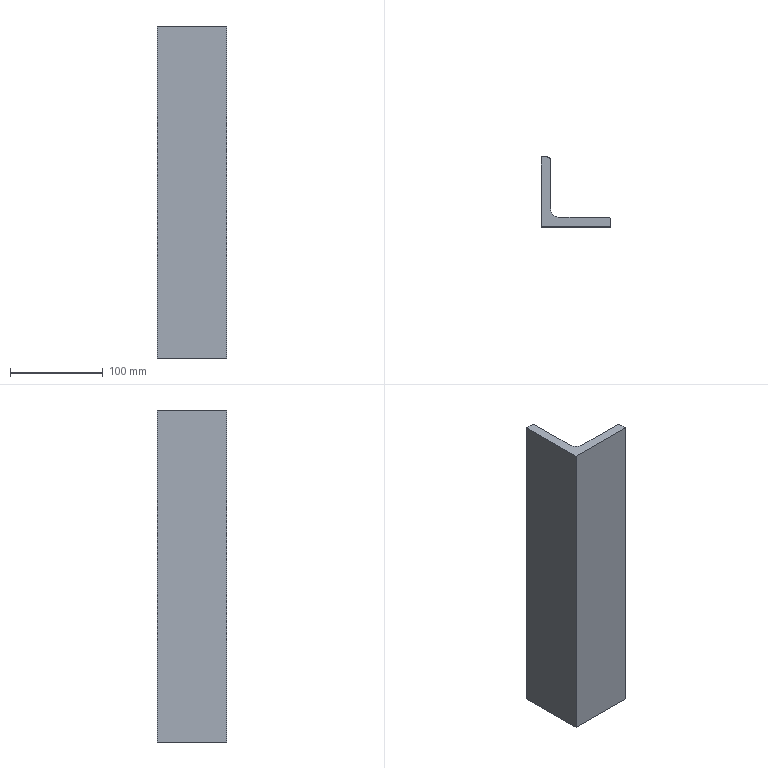Part | SolidWorks | features Extrusion 1 | 1 solid | 11 faces | box 75 x 75 x 358.1 mm | volume 505682 mm3 | plane 8 | cylinder 3 | commonest cylinder face diameters 7 x2 18 x1
STEP:
#1=CARTESIAN_POINT('',(6.5,75.,-179.05));
#2=VERTEX_POINT('',#1);
#3=CARTESIAN_POINT('',(0.,75.,-179.05));
#4=VERTEX_POINT('',#3);
#5=CARTESIAN_POINT('',(6.5,75.,-179.05));
#6=DIRECTION('',(-1.,0.,0.));
#7=VECTOR('',#6,1000.);
#8=LINE('',#5,#7);
#9=EDGE_CURVE('',#2,#4,#8,.T.);
#10=ORIENTED_EDGE('',*,*,#9,.T.);
#11=CARTESIAN_POINT('',(0.,75.,179.05));
#12=VERTEX_POINT('',#11);
#13=CARTESIAN_POINT('',(0.,75.,179.05));
#14=DIRECTION('',(0.,0.,-1.));
#15=VECTOR('',#14,1000.);
#16=LINE('',#13,#15);
#17=EDGE_CURVE('',#12,#4,#16,.T.);
#18=ORIENTED_EDGE('',*,*,#17,.F.);
#19=CARTESIAN_POINT('',(6.5,75.,179.05));
#20=VERTEX_POINT('',#19);
#21=CARTESIAN_POINT('',(6.5,75.,179.05));
#22=DIRECTION('',(-1.,0.,0.));
#23=VECTOR('',#22,1000.);
#24=LINE('',#21,#23);
#25=EDGE_CURVE('',#20,#12,#24,.T.);
#26=ORIENTED_EDGE('',*,*,#25,.F.);
#27=CARTESIAN_POINT('',(6.5,75.,179.05));
#28=DIRECTION('',(0.,0.,-1.));
#29=VECTOR('',#28,1000.);
#30=LINE('',#27,#29);
#31=EDGE_CURVE('',#20,#2,#30,.T.);
#32=ORIENTED_EDGE('',*,*,#31,.T.);
#33=EDGE_LOOP('',(#10,#18,#26,#32));
#34=FACE_OUTER_BOUND('',#33,.T.);
#35=CARTESIAN_POINT('',(6.5,75.,179.05));
#36=DIRECTION('',(0.,-1.,0.));
#37=DIRECTION('',(0.,0.,-1.));
#38=AXIS2_PLACEMENT_3D('',#35,#36,#37);
#39=PLANE('',#38);
#40=ADVANCED_FACE('',(#34),#39,.F.);
#41=CARTESIAN_POINT('',(0.,0.,-179.05));
#42=VERTEX_POINT('',#41);
#43=CARTESIAN_POINT('',(0.,75.,-179.05));
#44=DIRECTION('',(0.,-1.,0.));
#45=VECTOR('',#44,1000.);
#46=LINE('',#43,#45);
#47=EDGE_CURVE('',#4,#42,#46,.T.);
#48=ORIENTED_EDGE('',*,*,#47,.T.);
#49=CARTESIAN_POINT('',(0.,0.,179.05));
#50=VERTEX_POINT('',#49);
#51=CARTESIAN_POINT('',(0.,0.,179.05));
#52=DIRECTION('',(0.,0.,-1.));
#53=VECTOR('',#52,1000.);
#54=LINE('',#51,#53);
#55=EDGE_CURVE('',#50,#42,#54,.T.);
#56=ORIENTED_EDGE('',*,*,#55,.F.);
#57=CARTESIAN_POINT('',(0.,75.,179.05));
#58=DIRECTION('',(0.,-1.,0.));
#59=VECTOR('',#58,1000.);
#60=LINE('',#57,#59);
#61=EDGE_CURVE('',#12,#50,#60,.T.);
#62=ORIENTED_EDGE('',*,*,#61,.F.);
#63=ORIENTED_EDGE('',*,*,#17,.T.);
#64=EDGE_LOOP('',(#48,#56,#62,#63));
#65=FACE_OUTER_BOUND('',#64,.T.);
#66=CARTESIAN_POINT('',(0.,75.,179.05));
#67=DIRECTION('',(1.,0.,0.));
#68=DIRECTION('',(0.,1.,0.));
#69=AXIS2_PLACEMENT_3D('',#66,#67,#68);
#70=PLANE('',#69);
#71=ADVANCED_FACE('',(#65),#70,.F.);
#72=CARTESIAN_POINT('',(75.,0.,-179.05));
#73=VERTEX_POINT('',#72);
#74=CARTESIAN_POINT('',(0.,0.,-179.05));
#75=DIRECTION('',(1.,0.,0.));
#76=VECTOR('',#75,1000.);
#77=LINE('',#74,#76);
#78=EDGE_CURVE('',#42,#73,#77,.T.);
#79=ORIENTED_EDGE('',*,*,#78,.T.);
#80=CARTESIAN_POINT('',(75.,0.,179.05));
#81=VERTEX_POINT('',#80);
#82=CARTESIAN_POINT('',(75.,0.,179.05));
#83=DIRECTION('',(0.,0.,-1.));
#84=VECTOR('',#83,1000.);
#85=LINE('',#82,#84);
#86=EDGE_CURVE('',#81,#73,#85,.T.);
#87=ORIENTED_EDGE('',*,*,#86,.F.);
#88=CARTESIAN_POINT('',(0.,0.,179.05));
#89=DIRECTION('',(1.,0.,0.));
#90=VECTOR('',#89,1000.);
#91=LINE('',#88,#90);
#92=EDGE_CURVE('',#50,#81,#91,.T.);
#93=ORIENTED_EDGE('',*,*,#92,.F.);
#94=ORIENTED_EDGE('',*,*,#55,.T.);
#95=EDGE_LOOP('',(#79,#87,#93,#94));
#96=FACE_OUTER_BOUND('',#95,.T.);
#97=CARTESIAN_POINT('',(0.,0.,179.05));
#98=DIRECTION('',(0.,1.,0.));
#99=DIRECTION('',(0.,0.,1.));
#100=AXIS2_PLACEMENT_3D('',#97,#98,#99);
#101=PLANE('',#100);
#102=ADVANCED_FACE('',(#96),#101,.F.);
#103=CARTESIAN_POINT('',(75.,6.5,-179.05));
#104=VERTEX_POINT('',#103);
#105=CARTESIAN_POINT('',(75.,0.,-179.05));
#106=DIRECTION('',(0.,1.,0.));
#107=VECTOR('',#106,1000.);
#108=LINE('',#105,#107);
#109=EDGE_CURVE('',#73,#104,#108,.T.);
#110=ORIENTED_EDGE('',*,*,#109,.T.);
#111=CARTESIAN_POINT('',(75.,6.5,179.05));
#112=VERTEX_POINT('',#111);
#113=CARTESIAN_POINT('',(75.,6.5,179.05));
#114=DIRECTION('',(0.,0.,-1.));
#115=VECTOR('',#114,1000.);
#116=LINE('',#113,#115);
#117=EDGE_CURVE('',#112,#104,#116,.T.);
#118=ORIENTED_EDGE('',*,*,#117,.F.);
#119=CARTESIAN_POINT('',(75.,0.,179.05));
#120=DIRECTION('',(0.,1.,0.));
#121=VECTOR('',#120,1000.);
#122=LINE('',#119,#121);
#123=EDGE_CURVE('',#81,#112,#122,.T.);
#124=ORIENTED_EDGE('',*,*,#123,.F.);
#125=ORIENTED_EDGE('',*,*,#86,.T.);
#126=EDGE_LOOP('',(#110,#118,#124,#125));
#127=FACE_OUTER_BOUND('',#126,.T.);
#128=CARTESIAN_POINT('',(75.,0.,179.05));
#129=DIRECTION('',(-1.,0.,0.));
#130=DIRECTION('',(0.,0.,1.));
#131=AXIS2_PLACEMENT_3D('',#128,#129,#130);
#132=PLANE('',#131);
#133=ADVANCED_FACE('',(#127),#132,.F.);
#134=CARTESIAN_POINT('',(71.5,10.,-179.05));
#135=VERTEX_POINT('',#134);
#136=CARTESIAN_POINT('',(71.5,6.5,-179.05));
#137=DIRECTION('',(0.,0.,1.));
#138=DIRECTION('',(1.,0.,0.));
#139=AXIS2_PLACEMENT_3D('',#136,#137,#138);
#140=CIRCLE('',#139,3.5);
#141=EDGE_CURVE('',#104,#135,#140,.T.);
#142=ORIENTED_EDGE('',*,*,#141,.T.);
#143=CARTESIAN_POINT('',(71.5,10.,179.05));
#144=VERTEX_POINT('',#143);
#145=CARTESIAN_POINT('',(71.5,10.,179.05));
#146=DIRECTION('',(0.,0.,-1.));
#147=VECTOR('',#146,1000.);
#148=LINE('',#145,#147);
#149=EDGE_CURVE('',#144,#135,#148,.T.);
#150=ORIENTED_EDGE('',*,*,#149,.F.);
#151=CARTESIAN_POINT('',(71.5,6.5,179.05));
#152=DIRECTION('',(0.,0.,1.));
#153=DIRECTION('',(1.,0.,0.));
#154=AXIS2_PLACEMENT_3D('',#151,#152,#153);
#155=CIRCLE('',#154,3.5);
#156=EDGE_CURVE('',#112,#144,#155,.T.);
#157=ORIENTED_EDGE('',*,*,#156,.F.);
#158=ORIENTED_EDGE('',*,*,#117,.T.);
#159=EDGE_LOOP('',(#142,#150,#157,#158));
#160=FACE_OUTER_BOUND('',#159,.T.);
#161=CARTESIAN_POINT('',(71.5,6.5,179.05));
#162=DIRECTION('',(0.,0.,-1.));
#163=DIRECTION('',(-1.,0.,0.));
#164=AXIS2_PLACEMENT_3D('',#161,#162,#163);
#165=CYLINDRICAL_SURFACE('',#164,3.5);
#166=ADVANCED_FACE('',(#160),#165,.T.);
#167=CARTESIAN_POINT('',(19.,10.,-179.05));
#168=VERTEX_POINT('',#167);
#169=CARTESIAN_POINT('',(71.5,10.,-179.05));
#170=DIRECTION('',(-1.,0.,0.));
#171=VECTOR('',#170,1000.);
#172=LINE('',#169,#171);
#173=EDGE_CURVE('',#135,#168,#172,.T.);
#174=ORIENTED_EDGE('',*,*,#173,.T.);
#175=CARTESIAN_POINT('',(19.,10.,179.05));
#176=VERTEX_POINT('',#175);
#177=CARTESIAN_POINT('',(19.,10.,179.05));
#178=DIRECTION('',(0.,0.,-1.));
#179=VECTOR('',#178,1000.);
#180=LINE('',#177,#179);
#181=EDGE_CURVE('',#176,#168,#180,.T.);
#182=ORIENTED_EDGE('',*,*,#181,.F.);
#183=CARTESIAN_POINT('',(71.5,10.,179.05));
#184=DIRECTION('',(-1.,0.,0.));
#185=VECTOR('',#184,1000.);
#186=LINE('',#183,#185);
#187=EDGE_CURVE('',#144,#176,#186,.T.);
#188=ORIENTED_EDGE('',*,*,#187,.F.);
#189=ORIENTED_EDGE('',*,*,#149,.T.);
#190=EDGE_LOOP('',(#174,#182,#188,#189));
#191=FACE_OUTER_BOUND('',#190,.T.);
#192=CARTESIAN_POINT('',(71.5,10.,179.05));
#193=DIRECTION('',(0.,-1.,0.));
#194=DIRECTION('',(1.,0.,0.));
#195=AXIS2_PLACEMENT_3D('',#192,#193,#194);
#196=PLANE('',#195);
#197=ADVANCED_FACE('',(#191),#196,.F.);
#198=CARTESIAN_POINT('',(10.,19.,-179.05));
#199=VERTEX_POINT('',#198);
#200=CARTESIAN_POINT('',(19.,19.,-179.05));
#201=DIRECTION('',(0.,0.,-1.));
#202=DIRECTION('',(-1.,0.,0.));
#203=AXIS2_PLACEMENT_3D('',#200,#201,#202);
#204=CIRCLE('',#203,9.);
#205=EDGE_CURVE('',#168,#199,#204,.T.);
#206=ORIENTED_EDGE('',*,*,#205,.T.);
#207=CARTESIAN_POINT('',(10.,19.,179.05));
#208=VERTEX_POINT('',#207);
#209=CARTESIAN_POINT('',(10.,19.,179.05));
#210=DIRECTION('',(0.,0.,-1.));
#211=VECTOR('',#210,1000.);
#212=LINE('',#209,#211);
#213=EDGE_CURVE('',#208,#199,#212,.T.);
#214=ORIENTED_EDGE('',*,*,#213,.F.);
#215=CARTESIAN_POINT('',(19.,19.,179.05));
#216=DIRECTION('',(0.,0.,-1.));
#217=DIRECTION('',(-1.,0.,0.));
#218=AXIS2_PLACEMENT_3D('',#215,#216,#217);
#219=CIRCLE('',#218,9.);
#220=EDGE_CURVE('',#176,#208,#219,.T.);
#221=ORIENTED_EDGE('',*,*,#220,.F.);
#222=ORIENTED_EDGE('',*,*,#181,.T.);
#223=EDGE_LOOP('',(#206,#214,#221,#222));
#224=FACE_OUTER_BOUND('',#223,.T.);
#225=CARTESIAN_POINT('',(19.,19.,179.05));
#226=DIRECTION('',(0.,0.,-1.));
#227=DIRECTION('',(-1.,0.,0.));
#228=AXIS2_PLACEMENT_3D('',#225,#226,#227);
#229=CYLINDRICAL_SURFACE('',#228,9.);
#230=ADVANCED_FACE('',(#224),#229,.F.);
#231=CARTESIAN_POINT('',(10.,71.5,-179.05));
#232=VERTEX_POINT('',#231);
#233=CARTESIAN_POINT('',(10.,19.,-179.05));
#234=DIRECTION('',(0.,1.,0.));
#235=VECTOR('',#234,1000.);
#236=LINE('',#233,#235);
#237=EDGE_CURVE('',#199,#232,#236,.T.);
#238=ORIENTED_EDGE('',*,*,#237,.T.);
#239=CARTESIAN_POINT('',(10.,71.5,179.05));
#240=VERTEX_POINT('',#239);
#241=CARTESIAN_POINT('',(10.,71.5,179.05));
#242=DIRECTION('',(0.,0.,-1.));
#243=VECTOR('',#242,1000.);
#244=LINE('',#241,#243);
#245=EDGE_CURVE('',#240,#232,#244,.T.);
#246=ORIENTED_EDGE('',*,*,#245,.F.);
#247=CARTESIAN_POINT('',(10.,19.,179.05));
#248=DIRECTION('',(0.,1.,0.));
#249=VECTOR('',#248,1000.);
#250=LINE('',#247,#249);
#251=EDGE_CURVE('',#208,#240,#250,.T.);
#252=ORIENTED_EDGE('',*,*,#251,.F.);
#253=ORIENTED_EDGE('',*,*,#213,.T.);
#254=EDGE_LOOP('',(#238,#246,#252,#253));
#255=FACE_OUTER_BOUND('',#254,.T.);
#256=CARTESIAN_POINT('',(10.,19.,179.05));
#257=DIRECTION('',(-1.,0.,0.));
#258=DIRECTION('',(0.,-1.,0.));
#259=AXIS2_PLACEMENT_3D('',#256,#257,#258);
#260=PLANE('',#259);
#261=ADVANCED_FACE('',(#255),#260,.F.);
#262=CARTESIAN_POINT('',(6.5,71.5,-179.05));
#263=DIRECTION('',(0.,0.,1.));
#264=DIRECTION('',(1.,0.,0.));
#265=AXIS2_PLACEMENT_3D('',#262,#263,#264);
#266=CIRCLE('',#265,3.5);
#267=EDGE_CURVE('',#232,#2,#266,.T.);
#268=ORIENTED_EDGE('',*,*,#267,.T.);
#269=ORIENTED_EDGE('',*,*,#31,.F.);
#270=CARTESIAN_POINT('',(6.5,71.5,179.05));
#271=DIRECTION('',(0.,0.,1.));
#272=DIRECTION('',(1.,0.,0.));
#273=AXIS2_PLACEMENT_3D('',#270,#271,#272);
#274=CIRCLE('',#273,3.5);
#275=EDGE_CURVE('',#240,#20,#274,.T.);
#276=ORIENTED_EDGE('',*,*,#275,.F.);
#277=ORIENTED_EDGE('',*,*,#245,.T.);
#278=EDGE_LOOP('',(#268,#269,#276,#277));
#279=FACE_OUTER_BOUND('',#278,.T.);
#280=CARTESIAN_POINT('',(6.5,71.5,179.05));
#281=DIRECTION('',(0.,0.,-1.));
#282=DIRECTION('',(-1.,0.,0.));
#283=AXIS2_PLACEMENT_3D('',#280,#281,#282);
#284=CYLINDRICAL_SURFACE('',#283,3.5);
#285=ADVANCED_FACE('',(#279),#284,.T.);
#286=ORIENTED_EDGE('',*,*,#25,.T.);
#287=ORIENTED_EDGE('',*,*,#61,.T.);
#288=ORIENTED_EDGE('',*,*,#92,.T.);
#289=ORIENTED_EDGE('',*,*,#123,.T.);
#290=ORIENTED_EDGE('',*,*,#156,.T.);
#291=ORIENTED_EDGE('',*,*,#187,.T.);
#292=ORIENTED_EDGE('',*,*,#220,.T.);
#293=ORIENTED_EDGE('',*,*,#251,.T.);
#294=ORIENTED_EDGE('',*,*,#275,.T.);
#295=EDGE_LOOP('',(#286,#287,#288,#289,#290,#291,#292,#293,#294));
#296=FACE_OUTER_BOUND('',#295,.T.);
#297=CARTESIAN_POINT('',(71.5,6.5,179.05));
#298=DIRECTION('',(0.,0.,1.));
#299=DIRECTION('',(1.,0.,0.));
#300=AXIS2_PLACEMENT_3D('',#297,#298,#299);
#301=PLANE('',#300);
#302=ADVANCED_FACE('',(#296),#301,.T.);
#303=ORIENTED_EDGE('',*,*,#9,.F.);
#304=ORIENTED_EDGE('',*,*,#267,.F.);
#305=ORIENTED_EDGE('',*,*,#237,.F.);
#306=ORIENTED_EDGE('',*,*,#205,.F.);
#307=ORIENTED_EDGE('',*,*,#173,.F.);
#308=ORIENTED_EDGE('',*,*,#141,.F.);
#309=ORIENTED_EDGE('',*,*,#109,.F.);
#310=ORIENTED_EDGE('',*,*,#78,.F.);
#311=ORIENTED_EDGE('',*,*,#47,.F.);
#312=EDGE_LOOP('',(#303,#304,#305,#306,#307,#308,#309,#310,#311));
#313=FACE_OUTER_BOUND('',#312,.T.);
#314=CARTESIAN_POINT('',(71.5,6.5,-179.05));
#315=DIRECTION('',(0.,0.,1.));
#316=DIRECTION('',(1.,0.,0.));
#317=AXIS2_PLACEMENT_3D('',#314,#315,#316);
#318=PLANE('',#317);
#319=ADVANCED_FACE('',(#313),#318,.F.);
#320=CLOSED_SHELL('',(#40,#71,#102,#133,#166,#197,#230,#261,#285,#302,#319));
#321=MANIFOLD_SOLID_BREP('',#320);
#322=CARTESIAN_POINT('',(0.,0.,0.));
#323=DIRECTION('',(0.,0.,1.));
#324=DIRECTION('',(1.,0.,0.));
#325=AXIS2_PLACEMENT_3D('',#322,#323,#324);
#326=(LENGTH_UNIT()NAMED_UNIT(*)SI_UNIT(.MILLI.,.METRE.));
#327=UNCERTAINTY_MEASURE_WITH_UNIT(LENGTH_MEASURE(0.00001),#326,'','');
#328=(NAMED_UNIT(*)PLANE_ANGLE_UNIT()SI_UNIT($,.RADIAN.));
#329=(NAMED_UNIT(*)SI_UNIT($,.STERADIAN.)SOLID_ANGLE_UNIT());
#330=(GEOMETRIC_REPRESENTATION_CONTEXT(3)GLOBAL_UNCERTAINTY_ASSIGNED_CONTEXT((#327))GLOBAL_UNIT_ASSIGNED_CONTEXT((#326,#328,#329))REPRESENTATION_CONTEXT('',''));
#331=ADVANCED_BREP_SHAPE_REPRESENTATION('',(#321,#325),#330);